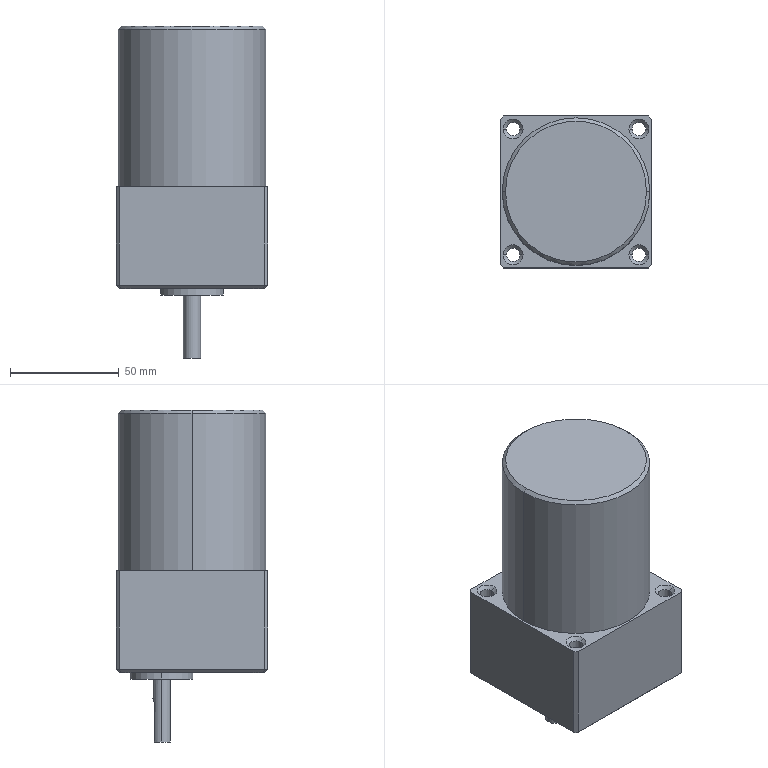Part | NX | features BREP 1 | 1 solid | 61 faces | box 70 x 70 x 153 mm | volume 495666 mm3 | plane 28 | cone 18 | cylinder 15 | commonest cylinder face diameters 6.2 x8 8 x2 29 x2 68 x2 4 x1